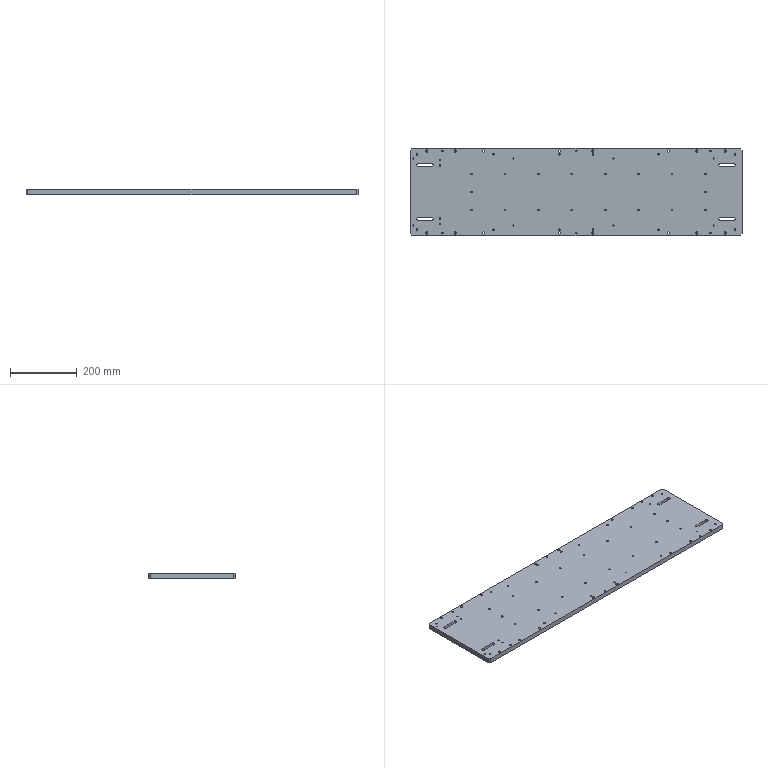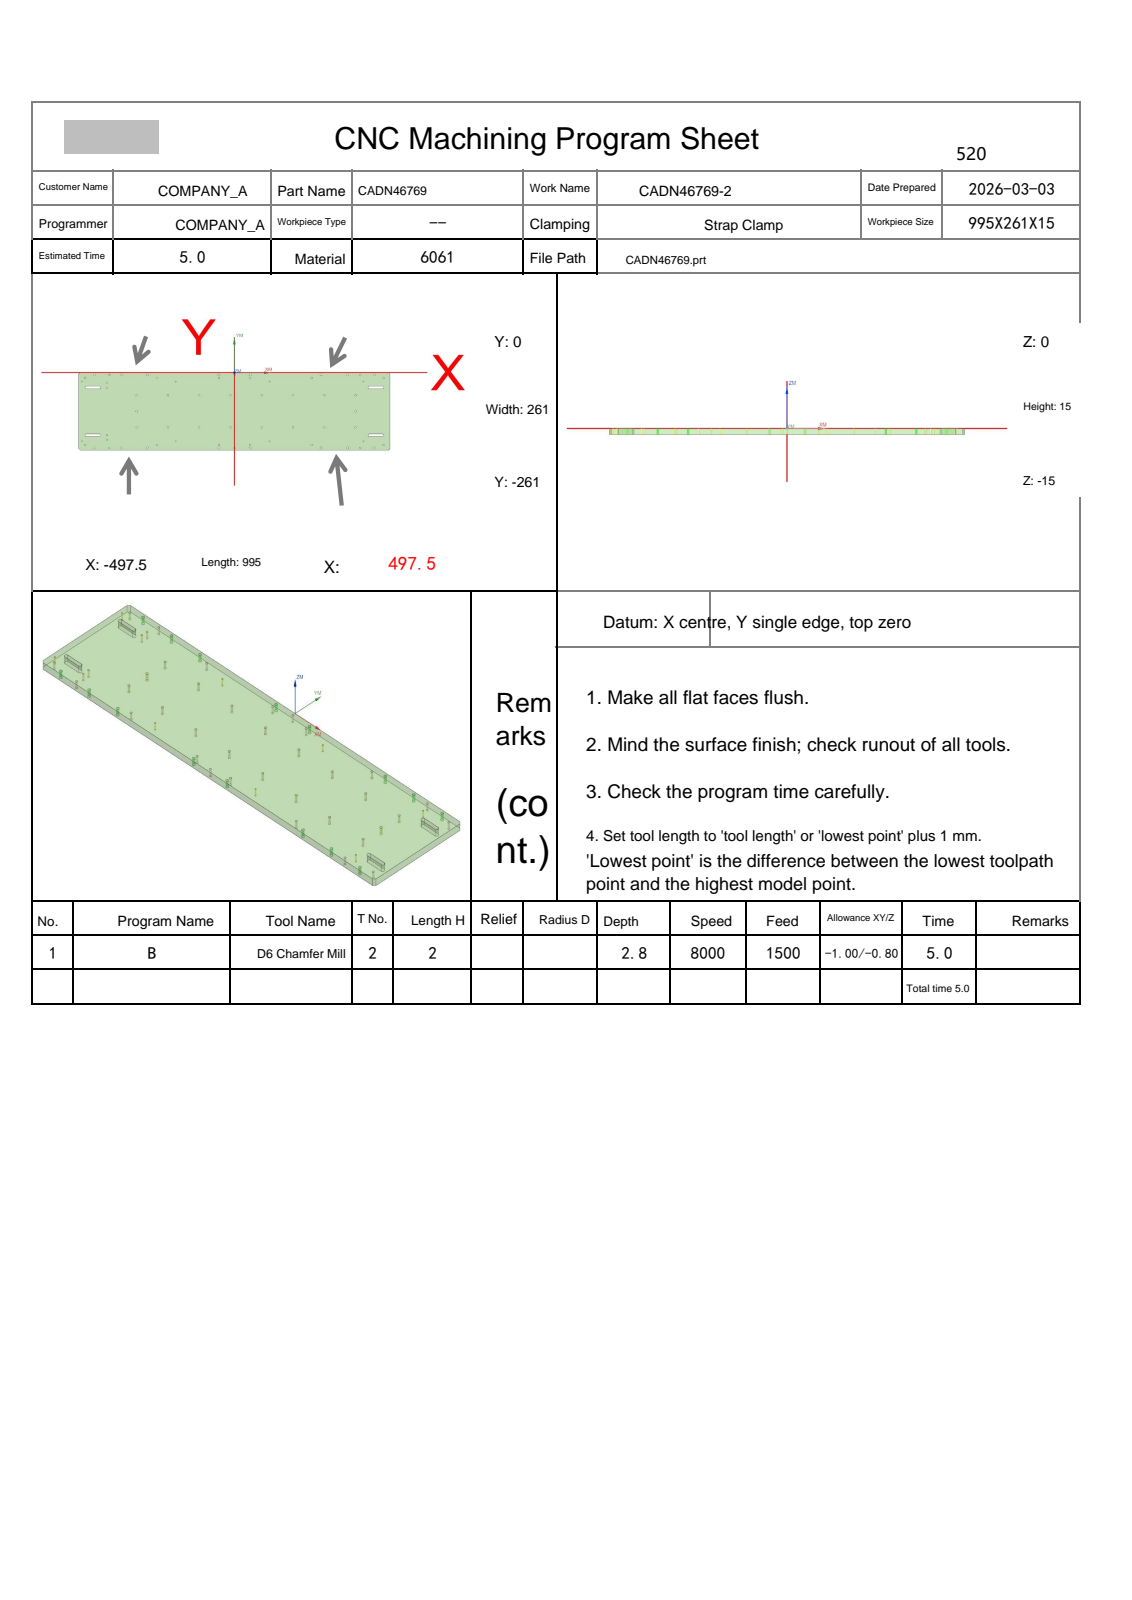NC program | NX | posted by the shop | part box 995 x 261 x 15 mm
Whole program:
%
O0001
(Machine time: 4.96 MIN)
(===Total Tool:1===)
(T2=D6 Chamfer Mill   D=6.   R=0.   D-  H02 Z=-2.8  )
G80 G90 G17 G49 G40
G91 G28 Z0
M01
N1 T02 M06
(D6 Chamfer Mill  D=6. R=0. H=02 ce=0.00 di=0.00)
G00 G90 G54 X-487.5 Y-231. M03 S3000
G43 H02 Z50.
M08
G98 G81 X-487.5 Y-231. Z-1.5 R1. F200.
X-477. Y-243.5
X-447. Y-253.5
X-407.5 Y-210.
Y-226.
X-400. Y-253.5
X-362.
X-312.5 Y-130.5
Y-184.5
X-277. Y-253.5
X-247. Y-243.5
X-212.5 Y-184.5
X-187.5 Y-231.
X-112.5 Y-184.5
X-12.5
X-49.5 Y-243.5
Y-253.5
X.5
X50.5
Y-243.5
X87.5 Y-184.5
X112.5 Y-231.
X187.5 Y-184.5
X247. Y-243.5
X277. Y-253.5
X287.5 Y-184.5
X362. Y-253.5
X402.5
X447.
X477. Y-243.5
X412.5 Y-231.
X387.5 Y-184.5
Y-130.5
Y-76.5
X412.5 Y-30.
X477. Y-17.5
X447. Y-7.5
X402.5
X362.
X277.
X247. Y-17.5
X287.5 Y-76.5
X187.5
X112.5 Y-30.
X87.5 Y-76.5
X50.5 Y-17.5
Y-7.5
X.5
X-49.5
Y-17.5
X-12.5 Y-76.5
X-112.5
X-187.5 Y-30.
X-212.5 Y-76.5
X-247. Y-17.5
X-277. Y-7.5
X-312.5 Y-76.5
X-362. Y-7.5
X-400.
X-407.5 Y-35.
Y-51.
X-447. Y-7.5
X-477. Y-17.5
X-487.5 Y-30.
G80
G00 Z50.
G00 G90 X387.227 Y-75.59 M03 S8000
Z50.
Z-.9
G01 Z-1.4 F600.
X387.05 Y-75.
G03 X385.55 Y-76.5 I0.0 J-1.5
X387.5 Y-78.45 I1.95 J0.0
X389.45 Y-76.5 I0.0 J1.95
X387.5 Y-74.55 I-1.95 J0.0
X385.55 Y-76.5 I0.0 J-1.95
X387.05 Y-78. I1.5 J0.0
G01 X387.227 Y-77.41
Z-.9
G00 Z50.
X287.227 Y-75.59
Z-.9
G01 Z-1.4
X287.05 Y-75.
G03 X285.55 Y-76.5 I0.0 J-1.5
X287.5 Y-78.45 I1.95 J0.0
X289.45 Y-76.5 I0.0 J1.95
X287.5 Y-74.55 I-1.95 J0.0
X285.55 Y-76.5 I0.0 J-1.95
X287.05 Y-78. I1.5 J0.0
G01 X287.227 Y-77.41
Z-.9
G00 Z50.
X187.227 Y-75.59
Z-.9
G01 Z-1.4
X187.05 Y-75.
G03 X185.55 Y-76.5 I0.0 J-1.5
X187.5 Y-78.45 I1.95 J0.0
X189.45 Y-76.5 I0.0 J1.95
X187.5 Y-74.55 I-1.95 J0.0
X185.55 Y-76.5 I0.0 J-1.95
X187.05 Y-78. I1.5 J0.0
G01 X187.227 Y-77.41
Z-.9
G00 Z50.
X87.227 Y-75.59
Z-.9
G01 Z-1.4
X87.05 Y-75.
G03 X85.55 Y-76.5 I0.0 J-1.5
X87.5 Y-78.45 I1.95 J0.0
X89.45 Y-76.5 I0.0 J1.95
X87.5 Y-74.55 I-1.95 J0.0
X85.55 Y-76.5 I0.0 J-1.95
X87.05 Y-78. I1.5 J0.0
G01 X87.227 Y-77.41
Z-.9
G00 Z50.
X-12.773 Y-75.59
Z-.9
G01 Z-1.4
X-12.95 Y-75.
G03 X-14.45 Y-76.5 I0.0 J-1.5
X-12.5 Y-78.45 I1.95 J0.0
X-10.55 Y-76.5 I0.0 J1.95
X-12.5 Y-74.55 I-1.95 J0.0
X-14.45 Y-76.5 I0.0 J-1.95
X-12.95 Y-78. I1.5 J0.0
G01 X-12.773 Y-77.41
Z-.9
G00 Z50.
X-112.773 Y-75.59
Z-.9
G01 Z-1.4
X-112.95 Y-75.
G03 X-114.45 Y-76.5 I0.0 J-1.5
X-112.5 Y-78.45 I1.95 J0.0
X-110.55 Y-76.5 I0.0 J1.95
X-112.5 Y-74.55 I-1.95 J0.0
X-114.45 Y-76.5 I0.0 J-1.95
X-112.95 Y-78. I1.5 J0.0
G01 X-112.773 Y-77.41
Z-.9
G00 Z50.
X-212.773 Y-75.59
Z-.9
G01 Z-1.4
X-212.95 Y-75.
G03 X-214.45 Y-76.5 I0.0 J-1.5
X-212.5 Y-78.45 I1.95 J0.0
X-210.55 Y-76.5 I0.0 J1.95
X-212.5 Y-74.55 I-1.95 J0.0
X-214.45 Y-76.5 I0.0 J-1.95
X-212.95 Y-78. I1.5 J0.0
G01 X-212.773 Y-77.41
Z-.9
G00 Z50.
X-312.773 Y-75.59
Z-.9
G01 Z-1.4
X-312.95 Y-75.
G03 X-314.45 Y-76.5 I0.0 J-1.5
X-312.5 Y-78.45 I1.95 J0.0
X-310.55 Y-76.5 I0.0 J1.95
X-312.5 Y-74.55 I-1.95 J0.0
X-314.45 Y-76.5 I0.0 J-1.95
X-312.95 Y-78. I1.5 J0.0
G01 X-312.773 Y-77.41
Z-.9
G00 Z50.
Y-183.59
Z-.9
G01 Z-1.4
X-312.95 Y-183.
G03 X-314.45 Y-184.5 I0.0 J-1.5
X-312.5 Y-186.45 I1.95 J0.0
X-310.55 Y-184.5 I0.0 J1.95
X-312.5 Y-182.55 I-1.95 J0.0
X-314.45 Y-184.5 I0.0 J-1.95
X-312.95 Y-186. I1.5 J0.0
G01 X-312.773 Y-185.41
Z-.9
G00 Z50.
X-212.773 Y-183.59
Z-.9
G01 Z-1.4
X-212.95 Y-183.
G03 X-214.45 Y-184.5 I0.0 J-1.5
X-212.5 Y-186.45 I1.95 J0.0
X-210.55 Y-184.5 I0.0 J1.95
X-212.5 Y-182.55 I-1.95 J0.0
X-214.45 Y-184.5 I0.0 J-1.95
X-212.95 Y-186. I1.5 J0.0
G01 X-212.773 Y-185.41
Z-.9
G00 Z50.
X-112.773 Y-183.59
Z-.9
G01 Z-1.4
X-112.95 Y-183.
G03 X-114.45 Y-184.5 I0.0 J-1.5
X-112.5 Y-186.45 I1.95 J0.0
X-110.55 Y-184.5 I0.0 J1.95
X-112.5 Y-182.55 I-1.95 J0.0
X-114.45 Y-184.5 I0.0 J-1.95
X-112.95 Y-186. I1.5 J0.0
G01 X-112.773 Y-185.41
Z-.9
G00 Z50.
X-12.773 Y-183.59
Z-.9
G01 Z-1.4
X-12.95 Y-183.
G03 X-14.45 Y-184.5 I0.0 J-1.5
X-12.5 Y-186.45 I1.95 J0.0
X-10.55 Y-184.5 I0.0 J1.95
X-12.5 Y-182.55 I-1.95 J0.0
X-14.45 Y-184.5 I0.0 J-1.95
X-12.95 Y-186. I1.5 J0.0
G01 X-12.773 Y-185.41
Z-.9
G00 Z50.
X87.227 Y-183.59
Z-.9
G01 Z-1.4
X87.05 Y-183.
G03 X85.55 Y-184.5 I0.0 J-1.5
X87.5 Y-186.45 I1.95 J0.0
X89.45 Y-184.5 I0.0 J1.95
X87.5 Y-182.55 I-1.95 J0.0
X85.55 Y-184.5 I0.0 J-1.95
X87.05 Y-186. I1.5 J0.0
G01 X87.227 Y-185.41
Z-.9
G00 Z50.
X187.227 Y-183.59
Z-.9
G01 Z-1.4
X187.05 Y-183.
G03 X185.55 Y-184.5 I0.0 J-1.5
X187.5 Y-186.45 I1.95 J0.0
X189.45 Y-184.5 I0.0 J1.95
X187.5 Y-182.55 I-1.95 J0.0
X185.55 Y-184.5 I0.0 J-1.95
X187.05 Y-186. I1.5 J0.0
G01 X187.227 Y-185.41
Z-.9
G00 Z50.
X287.227 Y-183.59
Z-.9
G01 Z-1.4
X287.05 Y-183.
G03 X285.55 Y-184.5 I0.0 J-1.5
X287.5 Y-186.45 I1.95 J0.0
X289.45 Y-184.5 I0.0 J1.95
X287.5 Y-182.55 I-1.95 J0.0
X285.55 Y-184.5 I0.0 J-1.95
X287.05 Y-186. I1.5 J0.0
G01 X287.227 Y-185.41
Z-.9
G00 Z50.
X387.227 Y-183.59
Z-.9
G01 Z-1.4
X387.05 Y-183.
G03 X385.55 Y-184.5 I0.0 J-1.5
X387.5 Y-186.45 I1.95 J0.0
X389.45 Y-184.5 I0.0 J1.95
X387.5 Y-182.55 I-1.95 J0.0
X385.55 Y-184.5 I0.0 J-1.95
X387.05 Y-186. I1.5 J0.0
G01 X387.227 Y-185.41
Z-.9
G00 Z50.
G00 G90 X-487.5 Y-30. M03 S8000
Z50.
G98 G81 X-487.5 Y-30. Z-2.2 R3. F1000.
Y-231.
X-187.5
Y-30.
X112.5
Y-231.
X412.5
Y-30.
G80
G00 Z50.
G00 G90 X-407.5 Y-35. M03 S8000
Z50.
G98 G81 X-407.5 Y-35. Z-2.7 R3. F1000.
Y-51.
Y-210.
Y-226.
G80
G00 Z50.
G00 G90 X477. Y-17.5 M03 S8000
Z50.
G98 G81 X477. Y-17.5 Z-2.8 R3. F1000.
X402.5 Y-7.5
X247. Y-17.5
X50.5
X.5 Y-7.5
X-49.5 Y-17.5
X-247.
X-400. Y-7.5
X-477. Y-17.5
Y-243.5
X-400. Y-253.5
X-247. Y-243.5
X-49.5
X.5 Y-253.5
X50.5 Y-243.5
X247.
X402.5 Y-253.5
X477. Y-243.5
G80
G00 Z50.
G00 G90 X-312.732 Y-129.63 M03 S8000
Z50.
Z-.9
G01 Z-1.4 F600.
X-312.9 Y-129.
G03 X-314.4 Y-130.5 I0.0 J-1.5
X-312.5 Y-132.4 I1.9 J0.0
X-310.6 Y-130.5 I0.0 J1.9
X-312.5 Y-128.6 I-1.9 J0.0
X-314.4 Y-130.5 I0.0 J-1.9
X-312.9 Y-132. I1.5 J0.0
G01 X-312.732 Y-131.37
Z-.9
G00 Z50.
X387.268 Y-129.63
Z-.9
G01 Z-1.4
X387.1 Y-129.
G03 X385.6 Y-130.5 I0.0 J-1.5
X387.5 Y-132.4 I1.9 J0.0
X389.4 Y-130.5 I0.0 J1.9
X387.5 Y-128.6 I-1.9 J0.0
X385.6 Y-130.5 I0.0 J-1.9
X387.1 Y-132. I1.5 J0.0
G01 X387.268 Y-131.37
Z-.9
G00 Z50.
G00 G90 X447. Y-251.5 M03 S8000
Z50.
Z-.9
G01 Z-1.4 F600.
Y-250.5
G03 X444. Y-253.5 I0.0 J-3.
X447. Y-256.5 I3. J0.0
X450. Y-253.5 I0.0 J3.
X447. Y-250.5 I-3. J0.0
X444. Y-253.5 I0.0 J-3.
X447. Y-256.5 I3. J0.0
G01 Y-255.5
Z-.9
G00 Z50.
X362. Y-251.5
Z-.9
G01 Z-1.4
Y-250.5
G03 X359. Y-253.5 I0.0 J-3.
X362. Y-256.5 I3. J0.0
X365. Y-253.5 I0.0 J3.
X362. Y-250.5 I-3. J0.0
X359. Y-253.5 I0.0 J-3.
X362. Y-256.5 I3. J0.0
G01 Y-255.5
Z-.9
G00 Z50.
X277. Y-251.5
Z-.9
G01 Z-1.4
Y-250.5
G03 X274. Y-253.5 I0.0 J-3.
X277. Y-256.5 I3. J0.0
X280. Y-253.5 I0.0 J3.
X277. Y-250.5 I-3. J0.0
X274. Y-253.5 I0.0 J-3.
X277. Y-256.5 I3. J0.0
G01 Y-255.5
Z-.9
G00 Z50.
X50.5 Y-251.5
Z-.9
G01 Z-1.4
Y-250.5
G03 X47.5 Y-253.5 I0.0 J-3.
X50.5 Y-256.5 I3. J0.0
X53.5 Y-253.5 I0.0 J3.
X50.5 Y-250.5 I-3. J0.0
X47.5 Y-253.5 I0.0 J-3.
X50.5 Y-256.5 I3. J0.0
G01 Y-255.5
Z-.9
G00 Z50.
X-49.5 Y-251.5
Z-.9
G01 Z-1.4
Y-250.5
G03 X-52.5 Y-253.5 I0.0 J-3.
X-49.5 Y-256.5 I3. J0.0
X-46.5 Y-253.5 I0.0 J3.
X-49.5 Y-250.5 I-3. J0.0
X-52.5 Y-253.5 I0.0 J-3.
X-49.5 Y-256.5 I3. J0.0
G01 Y-255.5
Z-.9
G00 Z50.
X-277. Y-251.5
Z-.9
G01 Z-1.4
Y-250.5
G03 X-280. Y-253.5 I0.0 J-3.
X-277. Y-256.5 I3. J0.0
X-274. Y-253.5 I0.0 J3.
X-277. Y-250.5 I-3. J0.0
X-280. Y-253.5 I0.0 J-3.
X-277. Y-256.5 I3. J0.0
G01 Y-255.5
Z-.9
G00 Z50.
X-362. Y-251.5
Z-.9
G01 Z-1.4
Y-250.5
G03 X-365. Y-253.5 I0.0 J-3.
X-362. Y-256.5 I3. J0.0
X-359. Y-253.5 I0.0 J3.
X-362. Y-250.5 I-3. J0.0
X-365. Y-253.5 I0.0 J-3.
X-362. Y-256.5 I3. J0.0
G01 Y-255.5
Z-.9
G00 Z50.
X-447. Y-251.5
Z-.9
G01 Z-1.4
Y-250.5
G03 X-450. Y-253.5 I0.0 J-3.
X-447. Y-256.5 I3. J0.0
X-444. Y-253.5 I0.0 J3.
X-447. Y-250.5 I-3. J0.0
X-450. Y-253.5 I0.0 J-3.
X-447. Y-256.5 I3. J0.0
G01 Y-255.5
Z-.9
G00 Z50.
Y-5.5
Z-.9
G01 Z-1.4
Y-4.5
G03 X-450. Y-7.5 I0.0 J-3.
X-447. Y-10.5 I3. J0.0
X-444. Y-7.5 I0.0 J3.
X-447. Y-4.5 I-3. J0.0
X-450. Y-7.5 I0.0 J-3.
X-447. Y-10.5 I3. J0.0
G01 Y-9.5
Z-.9
G00 Z50.
X-362. Y-5.5
Z-.9
G01 Z-1.4
Y-4.5
G03 X-365. Y-7.5 I0.0 J-3.
X-362. Y-10.5 I3. J0.0
X-359. Y-7.5 I0.0 J3.
X-362. Y-4.5 I-3. J0.0
X-365. Y-7.5 I0.0 J-3.
X-362. Y-10.5 I3. J0.0
G01 Y-9.5
Z-.9
G00 Z50.
X-277. Y-5.5
Z-.9
G01 Z-1.4
Y-4.5
G03 X-280. Y-7.5 I0.0 J-3.
X-277. Y-10.5 I3. J0.0
X-274. Y-7.5 I0.0 J3.
X-277. Y-4.5 I-3. J0.0
X-280. Y-7.5 I0.0 J-3.
X-277. Y-10.5 I3. J0.0
G01 Y-9.5
Z-.9
G00 Z50.
X-49.5 Y-5.5
Z-.9
G01 Z-1.4
Y-4.5
G03 X-52.5 Y-7.5 I0.0 J-3.
X-49.5 Y-10.5 I3. J0.0
X-46.5 Y-7.5 I0.0 J3.
X-49.5 Y-4.5 I-3. J0.0
X-52.5 Y-7.5 I0.0 J-3.
X-49.5 Y-10.5 I3. J0.0
G01 Y-9.5
Z-.9
G00 Z50.
X50.5 Y-5.5
Z-.9
G01 Z-1.4
Y-4.5
G03 X47.5 Y-7.5 I0.0 J-3.
X50.5 Y-10.5 I3. J0.0
X53.5 Y-7.5 I0.0 J3.
X50.5 Y-4.5 I-3. J0.0
X47.5 Y-7.5 I0.0 J-3.
X50.5 Y-10.5 I3. J0.0
G01 Y-9.5
Z-.9
G00 Z50.
X277. Y-5.5
Z-.9
G01 Z-1.4
Y-4.5
G03 X274. Y-7.5 I0.0 J-3.
X277. Y-10.5 I3. J0.0
X280. Y-7.5 I0.0 J3.
X277. Y-4.5 I-3. J0.0
X274. Y-7.5 I0.0 J-3.
X277. Y-10.5 I3. J0.0
G01 Y-9.5
Z-.9
G00 Z50.
X362. Y-5.5
Z-.9
G01 Z-1.4
Y-4.5
G03 X359. Y-7.5 I0.0 J-3.
X362. Y-10.5 I3. J0.0
X365. Y-7.5 I0.0 J3.
X362. Y-4.5 I-3. J0.0
X359. Y-7.5 I0.0 J-3.
X362. Y-10.5 I3. J0.0
G01 Y-9.5
Z-.9
G00 Z50.
X447. Y-5.5
Z-.9
G01 Z-1.4
Y-4.5
G03 X444. Y-7.5 I0.0 J-3.
X447. Y-10.5 I3. J0.0
X450. Y-7.5 I0.0 J3.
X447. Y-4.5 I-3. J0.0
X444. Y-7.5 I0.0 J-3.
X447. Y-10.5 I3. J0.0
G01 Y-9.5
Z-.9
G00 Z50.
G00 G90 X-463.384 Y-46.2 M03 S7000
Z50.
Z2.5
G01 X-473. Z-1. F1500.
G03 X-476.8 Y-50. I0.0 J-3.8
X-473. Y-53.8 I3.8 J0.0
G01 X-432.
G03 X-428.2 Y-50. I0.0 J3.8
X-432. Y-46.2 I-3.8 J0.0
G01 X-473.
G03 X-473.499 Y-46.233 I0.0 J-3.8
G01 Z1.5
G00 Z50.
X-463.384 Y-207.2
Z2.5
G01 X-473. Z-1.
G03 X-476.8 Y-211. I0.0 J-3.8
X-473. Y-214.8 I3.8 J0.0
G01 X-432.
G03 X-428.2 Y-211. I0.0 J3.8
X-432. Y-207.2 I-3.8 J0.0
G01 X-473.
G03 X-473.499 Y-207.233 I0.0 J-3.8
G01 Z1.5
G00 Z50.
X441.616 Y-207.2
Z2.5
G01 X432. Z-1.
G03 X428.2 Y-211. I0.0 J-3.8
X432. Y-214.8 I3.8 J0.0
G01 X473.
G03 X476.8 Y-211. I0.0 J3.8
X473. Y-207.2 I-3.8 J0.0
G01 X432.
G03 X431.501 Y-207.233 I0.0 J-3.8
G01 Z1.5
G00 Z50.
X441.616 Y-46.2
Z2.5
G01 X432. Z-1.
G03 X428.2 Y-50. I0.0 J-3.8
X432. Y-53.8 I3.8 J0.0
G01 X473.
G03 X476.8 Y-50. I0.0 J3.8
X473. Y-46.2 I-3.8 J0.0
G01 X432.
G03 X431.501 Y-46.233 I0.0 J-3.8
G01 Z1.5
G00 Z50.
G00 G90 X-490.874 Y-263.616 M03 S7000
Z50.
Z1.5
G01 Z-1. F1500.
X-492.995 Y-261.495
X-497.907 Y-256.583
G02 X-498.2 Y-255.876 I.707 J.707
G01 Y-5.124
G02 X-497.907 Y-4.417 I1. J0.0
G01 X-492.995 Y.495
X-490.874 Y2.616
Z1.5
G00 Z50.
X490.874
Z1.5
G01 Z-1.
X492.995 Y.495
X497.907 Y-4.417
G02 X498.2 Y-5.124 I-.707 J-.707
G01 Y-255.876
G02 X497.907 Y-256.583 I-1. J0.0
G01 X492.995 Y-261.495
X490.874 Y-263.616
Z1.5
G00 Z50.
M05
M09
G91 G28 Z0.0
G91 G28 Y0.0
M30
%